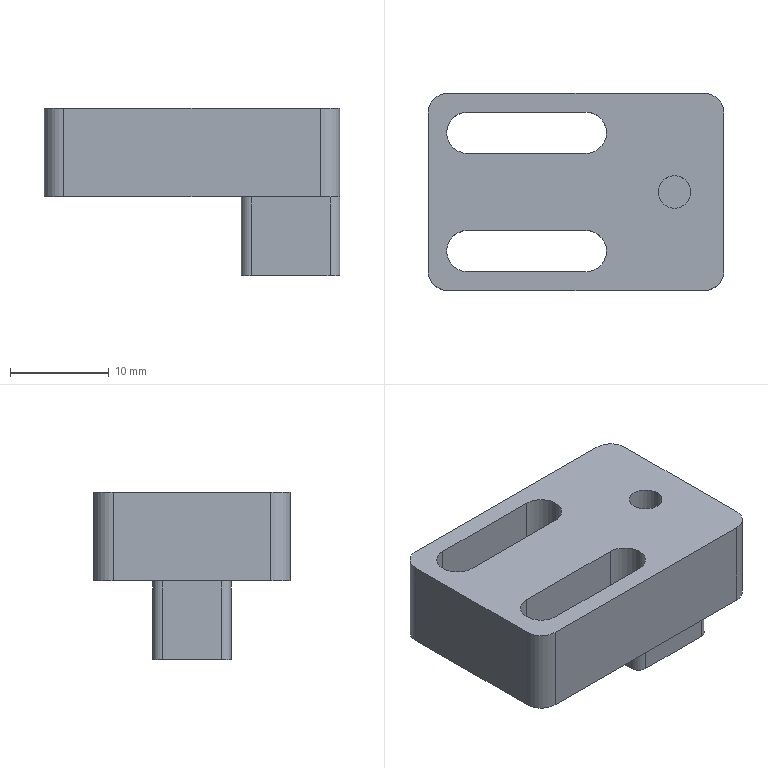Part | SolidWorks | features ICE 5, Fillet 3, Extrusion 1 | 1 solid | 31 faces | box 30 x 20 x 17 mm | volume 4794 mm3 | cylinder 16 | plane 15 | commonest cylinder face diameters 4.2 x6 2 x4 4 x4 3.3 x2
STEP:
#1=CARTESIAN_POINT('',(-9.,8.1,8.));
#2=VERTEX_POINT('',#1);
#3=CARTESIAN_POINT('',(-6.9,6.,8.));
#4=VERTEX_POINT('',#3);
#5=CARTESIAN_POINT('',(-9.,6.,8.));
#6=DIRECTION('',(0.,0.,-1.));
#7=DIRECTION('',(-1.,0.,0.));
#8=AXIS2_PLACEMENT_3D('',#5,#6,#7);
#9=CIRCLE('',#8,2.1);
#10=EDGE_CURVE('',#2,#4,#9,.T.);
#11=ORIENTED_EDGE('',*,*,#10,.T.);
#12=CARTESIAN_POINT('',(-6.9,6.,17.));
#13=VERTEX_POINT('',#12);
#14=CARTESIAN_POINT('',(-6.9,6.,-3.));
#15=DIRECTION('',(0.,0.,1.));
#16=VECTOR('',#15,1000.);
#17=LINE('',#14,#16);
#18=EDGE_CURVE('',#4,#13,#17,.T.);
#19=ORIENTED_EDGE('',*,*,#18,.T.);
#20=CARTESIAN_POINT('',(-9.,8.1,17.));
#21=VERTEX_POINT('',#20);
#22=CARTESIAN_POINT('',(-9.,6.,17.));
#23=DIRECTION('',(0.,0.,1.));
#24=DIRECTION('',(1.,0.,0.));
#25=AXIS2_PLACEMENT_3D('',#22,#23,#24);
#26=CIRCLE('',#25,2.1);
#27=EDGE_CURVE('',#13,#21,#26,.T.);
#28=ORIENTED_EDGE('',*,*,#27,.T.);
#29=CARTESIAN_POINT('',(-9.,8.1,-3.));
#30=DIRECTION('',(0.,0.,1.));
#31=VECTOR('',#30,1000.);
#32=LINE('',#29,#31);
#33=EDGE_CURVE('',#2,#21,#32,.T.);
#34=ORIENTED_EDGE('',*,*,#33,.F.);
#35=EDGE_LOOP('',(#11,#19,#28,#34));
#36=FACE_OUTER_BOUND('',#35,.T.);
#37=CARTESIAN_POINT('',(-9.,6.,-3.));
#38=DIRECTION('',(0.,0.,1.));
#39=DIRECTION('',(1.,0.,0.));
#40=AXIS2_PLACEMENT_3D('',#37,#38,#39);
#41=CYLINDRICAL_SURFACE('',#40,2.1);
#42=ADVANCED_FACE('',(#36),#41,.F.);
#43=CARTESIAN_POINT('',(-9.,-3.9,8.));
#44=VERTEX_POINT('',#43);
#45=CARTESIAN_POINT('',(-6.9,-6.,8.));
#46=VERTEX_POINT('',#45);
#47=CARTESIAN_POINT('',(-9.,-6.,8.));
#48=DIRECTION('',(0.,0.,-1.));
#49=DIRECTION('',(-1.,0.,0.));
#50=AXIS2_PLACEMENT_3D('',#47,#48,#49);
#51=CIRCLE('',#50,2.1);
#52=EDGE_CURVE('',#44,#46,#51,.T.);
#53=ORIENTED_EDGE('',*,*,#52,.T.);
#54=CARTESIAN_POINT('',(-6.9,-6.,17.));
#55=VERTEX_POINT('',#54);
#56=CARTESIAN_POINT('',(-6.9,-6.,-3.));
#57=DIRECTION('',(0.,0.,1.));
#58=VECTOR('',#57,1000.);
#59=LINE('',#56,#58);
#60=EDGE_CURVE('',#46,#55,#59,.T.);
#61=ORIENTED_EDGE('',*,*,#60,.T.);
#62=CARTESIAN_POINT('',(-9.,-3.9,17.));
#63=VERTEX_POINT('',#62);
#64=CARTESIAN_POINT('',(-9.,-6.,17.));
#65=DIRECTION('',(0.,0.,1.));
#66=DIRECTION('',(-1.,0.,0.));
#67=AXIS2_PLACEMENT_3D('',#64,#65,#66);
#68=CIRCLE('',#67,2.1);
#69=EDGE_CURVE('',#55,#63,#68,.T.);
#70=ORIENTED_EDGE('',*,*,#69,.T.);
#71=CARTESIAN_POINT('',(-9.,-3.9,-3.));
#72=DIRECTION('',(0.,0.,1.));
#73=VECTOR('',#72,1000.);
#74=LINE('',#71,#73);
#75=EDGE_CURVE('',#44,#63,#74,.T.);
#76=ORIENTED_EDGE('',*,*,#75,.F.);
#77=EDGE_LOOP('',(#53,#61,#70,#76));
#78=FACE_OUTER_BOUND('',#77,.T.);
#79=CARTESIAN_POINT('',(-9.,-6.,-3.));
#80=DIRECTION('',(0.,0.,1.));
#81=DIRECTION('',(1.,0.,0.));
#82=AXIS2_PLACEMENT_3D('',#79,#80,#81);
#83=CYLINDRICAL_SURFACE('',#82,2.1);
#84=ADVANCED_FACE('',(#78),#83,.F.);
#85=CARTESIAN_POINT('',(-1.65,0.,11.));
#86=VERTEX_POINT('',#85);
#87=CARTESIAN_POINT('',(1.65,0.,11.));
#88=VERTEX_POINT('',#87);
#89=CARTESIAN_POINT('',(0.,0.,11.));
#90=DIRECTION('',(0.,0.,1.));
#91=DIRECTION('',(1.,0.,0.));
#92=AXIS2_PLACEMENT_3D('',#89,#90,#91);
#93=CIRCLE('',#92,1.65);
#94=EDGE_CURVE('',#86,#88,#93,.T.);
#95=ORIENTED_EDGE('',*,*,#94,.F.);
#96=CARTESIAN_POINT('',(-1.65,0.,17.));
#97=VERTEX_POINT('',#96);
#98=CARTESIAN_POINT('',(-1.65,0.,11.));
#99=DIRECTION('',(0.,0.,1.));
#100=VECTOR('',#99,1000.);
#101=LINE('',#98,#100);
#102=EDGE_CURVE('',#86,#97,#101,.T.);
#103=ORIENTED_EDGE('',*,*,#102,.T.);
#104=CARTESIAN_POINT('',(1.65,0.,17.));
#105=VERTEX_POINT('',#104);
#106=CARTESIAN_POINT('',(0.,0.,17.));
#107=DIRECTION('',(0.,0.,1.));
#108=DIRECTION('',(1.,0.,0.));
#109=AXIS2_PLACEMENT_3D('',#106,#107,#108);
#110=CIRCLE('',#109,1.65);
#111=EDGE_CURVE('',#97,#105,#110,.T.);
#112=ORIENTED_EDGE('',*,*,#111,.T.);
#113=CARTESIAN_POINT('',(1.65,0.,11.));
#114=DIRECTION('',(0.,0.,1.));
#115=VECTOR('',#114,1000.);
#116=LINE('',#113,#115);
#117=EDGE_CURVE('',#88,#105,#116,.T.);
#118=ORIENTED_EDGE('',*,*,#117,.F.);
#119=EDGE_LOOP('',(#95,#103,#112,#118));
#120=FACE_OUTER_BOUND('',#119,.T.);
#121=CARTESIAN_POINT('',(0.,0.,11.));
#122=DIRECTION('',(0.,0.,1.));
#123=DIRECTION('',(1.,0.,0.));
#124=AXIS2_PLACEMENT_3D('',#121,#122,#123);
#125=CYLINDRICAL_SURFACE('',#124,1.65);
#126=ADVANCED_FACE('',(#120),#125,.F.);
#127=CARTESIAN_POINT('',(-5.,3.,8.));
#128=VERTEX_POINT('',#127);
#129=CARTESIAN_POINT('',(-5.,-3.,8.));
#130=VERTEX_POINT('',#129);
#131=CARTESIAN_POINT('',(-5.,10.,8.));
#132=DIRECTION('',(0.,-1.,0.));
#133=VECTOR('',#132,1000.);
#134=LINE('',#131,#133);
#135=EDGE_CURVE('',#128,#130,#134,.T.);
#136=ORIENTED_EDGE('',*,*,#135,.F.);
#137=CARTESIAN_POINT('',(-5.,3.,0.));
#138=VERTEX_POINT('',#137);
#139=CARTESIAN_POINT('',(-5.,3.,8.));
#140=DIRECTION('',(0.,0.,-1.));
#141=VECTOR('',#140,1000.);
#142=LINE('',#139,#141);
#143=EDGE_CURVE('',#128,#138,#142,.T.);
#144=ORIENTED_EDGE('',*,*,#143,.T.);
#145=CARTESIAN_POINT('',(-5.,-3.,0.));
#146=VERTEX_POINT('',#145);
#147=CARTESIAN_POINT('',(-5.,-4.,0.));
#148=DIRECTION('',(0.,-1.,0.));
#149=VECTOR('',#148,1000.);
#150=LINE('',#147,#149);
#151=EDGE_CURVE('',#138,#146,#150,.T.);
#152=ORIENTED_EDGE('',*,*,#151,.T.);
#153=CARTESIAN_POINT('',(-5.,-3.,8.));
#154=DIRECTION('',(0.,0.,1.));
#155=VECTOR('',#154,1000.);
#156=LINE('',#153,#155);
#157=EDGE_CURVE('',#146,#130,#156,.T.);
#158=ORIENTED_EDGE('',*,*,#157,.T.);
#159=EDGE_LOOP('',(#136,#144,#152,#158));
#160=FACE_OUTER_BOUND('',#159,.T.);
#161=CARTESIAN_POINT('',(-5.,-4.,8.));
#162=DIRECTION('',(1.,0.,0.));
#163=DIRECTION('',(0.,0.,-1.));
#164=AXIS2_PLACEMENT_3D('',#161,#162,#163);
#165=PLANE('',#164);
#166=ADVANCED_FACE('',(#160),#165,.F.);
#167=CARTESIAN_POINT('',(5.,-3.,0.));
#168=VERTEX_POINT('',#167);
#169=CARTESIAN_POINT('',(5.,3.,0.));
#170=VERTEX_POINT('',#169);
#171=CARTESIAN_POINT('',(5.,-4.,0.));
#172=DIRECTION('',(0.,1.,0.));
#173=VECTOR('',#172,1000.);
#174=LINE('',#171,#173);
#175=EDGE_CURVE('',#168,#170,#174,.T.);
#176=ORIENTED_EDGE('',*,*,#175,.T.);
#177=CARTESIAN_POINT('',(5.,3.,8.));
#178=VERTEX_POINT('',#177);
#179=CARTESIAN_POINT('',(5.,3.,8.));
#180=DIRECTION('',(0.,0.,1.));
#181=VECTOR('',#180,1000.);
#182=LINE('',#179,#181);
#183=EDGE_CURVE('',#170,#178,#182,.T.);
#184=ORIENTED_EDGE('',*,*,#183,.T.);
#185=CARTESIAN_POINT('',(5.,8.,8.));
#186=VERTEX_POINT('',#185);
#187=CARTESIAN_POINT('',(5.,-10.,8.));
#188=DIRECTION('',(0.,1.,0.));
#189=VECTOR('',#188,1000.);
#190=LINE('',#187,#189);
#191=EDGE_CURVE('',#178,#186,#190,.T.);
#192=ORIENTED_EDGE('',*,*,#191,.T.);
#193=CARTESIAN_POINT('',(5.,8.,17.));
#194=VERTEX_POINT('',#193);
#195=CARTESIAN_POINT('',(5.,8.,8.));
#196=DIRECTION('',(0.,0.,1.));
#197=VECTOR('',#196,1000.);
#198=LINE('',#195,#197);
#199=EDGE_CURVE('',#186,#194,#198,.T.);
#200=ORIENTED_EDGE('',*,*,#199,.T.);
#201=CARTESIAN_POINT('',(5.,-8.,17.));
#202=VERTEX_POINT('',#201);
#203=CARTESIAN_POINT('',(5.,-10.,17.));
#204=DIRECTION('',(0.,1.,0.));
#205=VECTOR('',#204,1000.);
#206=LINE('',#203,#205);
#207=EDGE_CURVE('',#202,#194,#206,.T.);
#208=ORIENTED_EDGE('',*,*,#207,.F.);
#209=CARTESIAN_POINT('',(5.,-8.,8.));
#210=VERTEX_POINT('',#209);
#211=CARTESIAN_POINT('',(5.,-8.,8.));
#212=DIRECTION('',(0.,0.,-1.));
#213=VECTOR('',#212,1000.);
#214=LINE('',#211,#213);
#215=EDGE_CURVE('',#202,#210,#214,.T.);
#216=ORIENTED_EDGE('',*,*,#215,.T.);
#217=CARTESIAN_POINT('',(5.,-3.,8.));
#218=VERTEX_POINT('',#217);
#219=CARTESIAN_POINT('',(5.,-10.,8.));
#220=DIRECTION('',(0.,1.,0.));
#221=VECTOR('',#220,1000.);
#222=LINE('',#219,#221);
#223=EDGE_CURVE('',#210,#218,#222,.T.);
#224=ORIENTED_EDGE('',*,*,#223,.T.);
#225=CARTESIAN_POINT('',(5.,-3.,8.));
#226=DIRECTION('',(0.,0.,-1.));
#227=VECTOR('',#226,1000.);
#228=LINE('',#225,#227);
#229=EDGE_CURVE('',#218,#168,#228,.T.);
#230=ORIENTED_EDGE('',*,*,#229,.T.);
#231=EDGE_LOOP('',(#176,#184,#192,#200,#208,#216,#224,#230));
#232=FACE_OUTER_BOUND('',#231,.T.);
#233=CARTESIAN_POINT('',(5.,-4.,8.));
#234=DIRECTION('',(-1.,0.,0.));
#235=DIRECTION('',(0.,0.,1.));
#236=AXIS2_PLACEMENT_3D('',#233,#234,#235);
#237=PLANE('',#236);
#238=ADVANCED_FACE('',(#232),#237,.F.);
#239=CARTESIAN_POINT('',(4.,4.,0.));
#240=VERTEX_POINT('',#239);
#241=CARTESIAN_POINT('',(-4.,4.,0.));
#242=VERTEX_POINT('',#241);
#243=CARTESIAN_POINT('',(-5.,4.,0.));
#244=DIRECTION('',(-1.,0.,0.));
#245=VECTOR('',#244,1000.);
#246=LINE('',#243,#245);
#247=EDGE_CURVE('',#240,#242,#246,.T.);
#248=ORIENTED_EDGE('',*,*,#247,.T.);
#249=CARTESIAN_POINT('',(-4.,4.,8.));
#250=VERTEX_POINT('',#249);
#251=CARTESIAN_POINT('',(-4.,4.,8.));
#252=DIRECTION('',(0.,0.,1.));
#253=VECTOR('',#252,1000.);
#254=LINE('',#251,#253);
#255=EDGE_CURVE('',#242,#250,#254,.T.);
#256=ORIENTED_EDGE('',*,*,#255,.T.);
#257=CARTESIAN_POINT('',(4.,4.,8.));
#258=VERTEX_POINT('',#257);
#259=CARTESIAN_POINT('',(-5.,4.,8.));
#260=DIRECTION('',(-1.,0.,0.));
#261=VECTOR('',#260,1000.);
#262=LINE('',#259,#261);
#263=EDGE_CURVE('',#258,#250,#262,.T.);
#264=ORIENTED_EDGE('',*,*,#263,.F.);
#265=CARTESIAN_POINT('',(4.,4.,8.));
#266=DIRECTION('',(0.,0.,-1.));
#267=VECTOR('',#266,1000.);
#268=LINE('',#265,#267);
#269=EDGE_CURVE('',#258,#240,#268,.T.);
#270=ORIENTED_EDGE('',*,*,#269,.T.);
#271=EDGE_LOOP('',(#248,#256,#264,#270));
#272=FACE_OUTER_BOUND('',#271,.T.);
#273=CARTESIAN_POINT('',(-5.,4.,8.));
#274=DIRECTION('',(0.,-1.,0.));
#275=DIRECTION('',(0.,0.,-1.));
#276=AXIS2_PLACEMENT_3D('',#273,#274,#275);
#277=PLANE('',#276);
#278=ADVANCED_FACE('',(#272),#277,.F.);
#279=CARTESIAN_POINT('',(-4.,-4.,0.));
#280=VERTEX_POINT('',#279);
#281=CARTESIAN_POINT('',(4.,-4.,0.));
#282=VERTEX_POINT('',#281);
#283=CARTESIAN_POINT('',(-5.,-4.,0.));
#284=DIRECTION('',(1.,0.,0.));
#285=VECTOR('',#284,1000.);
#286=LINE('',#283,#285);
#287=EDGE_CURVE('',#280,#282,#286,.T.);
#288=ORIENTED_EDGE('',*,*,#287,.T.);
#289=CARTESIAN_POINT('',(4.,-4.,8.));
#290=VERTEX_POINT('',#289);
#291=CARTESIAN_POINT('',(4.,-4.,8.));
#292=DIRECTION('',(0.,0.,1.));
#293=VECTOR('',#292,1000.);
#294=LINE('',#291,#293);
#295=EDGE_CURVE('',#282,#290,#294,.T.);
#296=ORIENTED_EDGE('',*,*,#295,.T.);
#297=CARTESIAN_POINT('',(-4.,-4.,8.));
#298=VERTEX_POINT('',#297);
#299=CARTESIAN_POINT('',(-5.,-4.,8.));
#300=DIRECTION('',(1.,0.,0.));
#301=VECTOR('',#300,1000.);
#302=LINE('',#299,#301);
#303=EDGE_CURVE('',#298,#290,#302,.T.);
#304=ORIENTED_EDGE('',*,*,#303,.F.);
#305=CARTESIAN_POINT('',(-4.,-4.,8.));
#306=DIRECTION('',(0.,0.,-1.));
#307=VECTOR('',#306,1000.);
#308=LINE('',#305,#307);
#309=EDGE_CURVE('',#298,#280,#308,.T.);
#310=ORIENTED_EDGE('',*,*,#309,.T.);
#311=EDGE_LOOP('',(#288,#296,#304,#310));
#312=FACE_OUTER_BOUND('',#311,.T.);
#313=CARTESIAN_POINT('',(-5.,-4.,8.));
#314=DIRECTION('',(0.,1.,0.));
#315=DIRECTION('',(0.,0.,1.));
#316=AXIS2_PLACEMENT_3D('',#313,#314,#315);
#317=PLANE('',#316);
#318=ADVANCED_FACE('',(#312),#317,.F.);
#319=ORIENTED_EDGE('',*,*,#151,.F.);
#320=CARTESIAN_POINT('',(-4.,3.,0.));
#321=DIRECTION('',(0.,0.,-1.));
#322=DIRECTION('',(-1.,0.,0.));
#323=AXIS2_PLACEMENT_3D('',#320,#321,#322);
#324=CIRCLE('',#323,1.);
#325=EDGE_CURVE('',#138,#242,#324,.T.);
#326=ORIENTED_EDGE('',*,*,#325,.T.);
#327=ORIENTED_EDGE('',*,*,#247,.F.);
#328=CARTESIAN_POINT('',(4.,3.,0.));
#329=DIRECTION('',(0.,0.,-1.));
#330=DIRECTION('',(-1.,0.,0.));
#331=AXIS2_PLACEMENT_3D('',#328,#329,#330);
#332=CIRCLE('',#331,1.);
#333=EDGE_CURVE('',#240,#170,#332,.T.);
#334=ORIENTED_EDGE('',*,*,#333,.T.);
#335=ORIENTED_EDGE('',*,*,#175,.F.);
#336=CARTESIAN_POINT('',(4.,-3.,0.));
#337=DIRECTION('',(0.,0.,-1.));
#338=DIRECTION('',(-1.,0.,0.));
#339=AXIS2_PLACEMENT_3D('',#336,#337,#338);
#340=CIRCLE('',#339,1.);
#341=EDGE_CURVE('',#168,#282,#340,.T.);
#342=ORIENTED_EDGE('',*,*,#341,.T.);
#343=ORIENTED_EDGE('',*,*,#287,.F.);
#344=CARTESIAN_POINT('',(-4.,-3.,0.));
#345=DIRECTION('',(0.,0.,-1.));
#346=DIRECTION('',(-1.,0.,0.));
#347=AXIS2_PLACEMENT_3D('',#344,#345,#346);
#348=CIRCLE('',#347,1.);
#349=EDGE_CURVE('',#280,#146,#348,.T.);
#350=ORIENTED_EDGE('',*,*,#349,.T.);
#351=EDGE_LOOP('',(#319,#326,#327,#334,#335,#342,#343,#350));
#352=FACE_OUTER_BOUND('',#351,.T.);
#353=CARTESIAN_POINT('',(0.,0.,0.));
#354=DIRECTION('',(0.,0.,-1.));
#355=DIRECTION('',(-1.,0.,0.));
#356=AXIS2_PLACEMENT_3D('',#353,#354,#355);
#357=PLANE('',#356);
#358=ADVANCED_FACE('',(#352),#357,.T.);
#359=CARTESIAN_POINT('',(-21.,3.9,8.));
#360=VERTEX_POINT('',#359);
#361=CARTESIAN_POINT('',(-21.,8.1,8.));
#362=VERTEX_POINT('',#361);
#363=CARTESIAN_POINT('',(-21.,6.,8.));
#364=DIRECTION('',(0.,0.,-1.));
#365=DIRECTION('',(-1.,0.,0.));
#366=AXIS2_PLACEMENT_3D('',#363,#364,#365);
#367=CIRCLE('',#366,2.1);
#368=EDGE_CURVE('',#360,#362,#367,.T.);
#369=ORIENTED_EDGE('',*,*,#368,.F.);
#370=CARTESIAN_POINT('',(-9.,3.9,8.));
#371=VERTEX_POINT('',#370);
#372=CARTESIAN_POINT('',(0.,3.9,8.));
#373=DIRECTION('',(-1.,0.,0.));
#374=VECTOR('',#373,1000.);
#375=LINE('',#372,#374);
#376=EDGE_CURVE('',#371,#360,#375,.T.);
#377=ORIENTED_EDGE('',*,*,#376,.F.);
#378=CARTESIAN_POINT('',(-9.,6.,8.));
#379=DIRECTION('',(0.,0.,-1.));
#380=DIRECTION('',(-1.,0.,0.));
#381=AXIS2_PLACEMENT_3D('',#378,#379,#380);
#382=CIRCLE('',#381,2.1);
#383=EDGE_CURVE('',#4,#371,#382,.T.);
#384=ORIENTED_EDGE('',*,*,#383,.F.);
#385=ORIENTED_EDGE('',*,*,#10,.F.);
#386=CARTESIAN_POINT('',(0.,8.1,8.));
#387=DIRECTION('',(1.,0.,0.));
#388=VECTOR('',#387,1000.);
#389=LINE('',#386,#388);
#390=EDGE_CURVE('',#362,#2,#389,.T.);
#391=ORIENTED_EDGE('',*,*,#390,.F.);
#392=EDGE_LOOP('',(#369,#377,#384,#385,#391));
#393=FACE_BOUND('',#392,.T.);
#394=CARTESIAN_POINT('',(-21.,-8.1,8.));
#395=VERTEX_POINT('',#394);
#396=CARTESIAN_POINT('',(-21.,-3.9,8.));
#397=VERTEX_POINT('',#396);
#398=CARTESIAN_POINT('',(-21.,-6.,8.));
#399=DIRECTION('',(0.,0.,-1.));
#400=DIRECTION('',(-1.,0.,0.));
#401=AXIS2_PLACEMENT_3D('',#398,#399,#400);
#402=CIRCLE('',#401,2.1);
#403=EDGE_CURVE('',#395,#397,#402,.T.);
#404=ORIENTED_EDGE('',*,*,#403,.F.);
#405=CARTESIAN_POINT('',(-9.,-8.1,8.));
#406=VERTEX_POINT('',#405);
#407=CARTESIAN_POINT('',(0.,-8.1,8.));
#408=DIRECTION('',(-1.,0.,0.));
#409=VECTOR('',#408,1000.);
#410=LINE('',#407,#409);
#411=EDGE_CURVE('',#406,#395,#410,.T.);
#412=ORIENTED_EDGE('',*,*,#411,.F.);
#413=CARTESIAN_POINT('',(-9.,-6.,8.));
#414=DIRECTION('',(0.,0.,-1.));
#415=DIRECTION('',(-1.,0.,0.));
#416=AXIS2_PLACEMENT_3D('',#413,#414,#415);
#417=CIRCLE('',#416,2.1);
#418=EDGE_CURVE('',#46,#406,#417,.T.);
#419=ORIENTED_EDGE('',*,*,#418,.F.);
#420=ORIENTED_EDGE('',*,*,#52,.F.);
#421=CARTESIAN_POINT('',(0.,-3.9,8.));
#422=DIRECTION('',(1.,0.,0.));
#423=VECTOR('',#422,1000.);
#424=LINE('',#421,#423);
#425=EDGE_CURVE('',#397,#44,#424,.T.);
#426=ORIENTED_EDGE('',*,*,#425,.F.);
#427=EDGE_LOOP('',(#404,#412,#419,#420,#426));
#428=FACE_BOUND('',#427,.T.);
#429=CARTESIAN_POINT('',(3.,10.,8.));
#430=VERTEX_POINT('',#429);
#431=CARTESIAN_POINT('',(-23.,10.,8.));
#432=VERTEX_POINT('',#431);
#433=CARTESIAN_POINT('',(-5.,10.,8.));
#434=DIRECTION('',(-1.,0.,0.));
#435=VECTOR('',#434,1000.);
#436=LINE('',#433,#435);
#437=EDGE_CURVE('',#430,#432,#436,.T.);
#438=ORIENTED_EDGE('',*,*,#437,.F.);
#439=CARTESIAN_POINT('',(3.,8.,8.));
#440=DIRECTION('',(0.,0.,-1.));
#441=DIRECTION('',(-1.,0.,0.));
#442=AXIS2_PLACEMENT_3D('',#439,#440,#441);
#443=CIRCLE('',#442,2.);
#444=EDGE_CURVE('',#430,#186,#443,.T.);
#445=ORIENTED_EDGE('',*,*,#444,.T.);
#446=ORIENTED_EDGE('',*,*,#191,.F.);
#447=CARTESIAN_POINT('',(4.,3.,8.));
#448=DIRECTION('',(0.,0.,1.));
#449=DIRECTION('',(-1.,0.,0.));
#450=AXIS2_PLACEMENT_3D('',#447,#448,#449);
#451=CIRCLE('',#450,1.);
#452=EDGE_CURVE('',#178,#258,#451,.T.);
#453=ORIENTED_EDGE('',*,*,#452,.T.);
#454=ORIENTED_EDGE('',*,*,#263,.T.);
#455=CARTESIAN_POINT('',(-4.,3.,8.));
#456=DIRECTION('',(0.,0.,1.));
#457=DIRECTION('',(-1.,0.,0.));
#458=AXIS2_PLACEMENT_3D('',#455,#456,#457);
#459=CIRCLE('',#458,1.);
#460=EDGE_CURVE('',#250,#128,#459,.T.);
#461=ORIENTED_EDGE('',*,*,#460,.T.);
#462=ORIENTED_EDGE('',*,*,#135,.T.);
#463=CARTESIAN_POINT('',(-4.,-3.,8.));
#464=DIRECTION('',(0.,0.,1.));
#465=DIRECTION('',(-1.,0.,0.));
#466=AXIS2_PLACEMENT_3D('',#463,#464,#465);
#467=CIRCLE('',#466,1.);
#468=EDGE_CURVE('',#130,#298,#467,.T.);
#469=ORIENTED_EDGE('',*,*,#468,.T.);
#470=ORIENTED_EDGE('',*,*,#303,.T.);
#471=CARTESIAN_POINT('',(4.,-3.,8.));
#472=DIRECTION('',(0.,0.,1.));
#473=DIRECTION('',(-1.,0.,0.));
#474=AXIS2_PLACEMENT_3D('',#471,#472,#473);
#475=CIRCLE('',#474,1.);
#476=EDGE_CURVE('',#290,#218,#475,.T.);
#477=ORIENTED_EDGE('',*,*,#476,.T.);
#478=ORIENTED_EDGE('',*,*,#223,.F.);
#479=CARTESIAN_POINT('',(3.,-10.,8.));
#480=VERTEX_POINT('',#479);
#481=CARTESIAN_POINT('',(3.,-8.,8.));
#482=DIRECTION('',(0.,0.,-1.));
#483=DIRECTION('',(-1.,0.,0.));
#484=AXIS2_PLACEMENT_3D('',#481,#482,#483);
#485=CIRCLE('',#484,2.);
#486=EDGE_CURVE('',#210,#480,#485,.T.);
#487=ORIENTED_EDGE('',*,*,#486,.T.);
#488=CARTESIAN_POINT('',(-23.,-10.,8.));
#489=VERTEX_POINT('',#488);
#490=CARTESIAN_POINT('',(-5.,-10.,8.));
#491=DIRECTION('',(1.,0.,0.));
#492=VECTOR('',#491,1000.);
#493=LINE('',#490,#492);
#494=EDGE_CURVE('',#489,#480,#493,.T.);
#495=ORIENTED_EDGE('',*,*,#494,.F.);
#496=CARTESIAN_POINT('',(-25.,-8.,8.));
#497=VERTEX_POINT('',#496);
#498=CARTESIAN_POINT('',(-23.,-8.,8.));
#499=DIRECTION('',(0.,0.,-1.));
#500=DIRECTION('',(-1.,0.,0.));
#501=AXIS2_PLACEMENT_3D('',#498,#499,#500);
#502=CIRCLE('',#501,2.);
#503=EDGE_CURVE('',#489,#497,#502,.T.);
#504=ORIENTED_EDGE('',*,*,#503,.T.);
#505=CARTESIAN_POINT('',(-25.,8.,8.));
#506=VERTEX_POINT('',#505);
#507=CARTESIAN_POINT('',(-25.,10.,8.));
#508=DIRECTION('',(0.,-1.,0.));
#509=VECTOR('',#508,1000.);
#510=LINE('',#507,#509);
#511=EDGE_CURVE('',#506,#497,#510,.T.);
#512=ORIENTED_EDGE('',*,*,#511,.F.);
#513=CARTESIAN_POINT('',(-23.,8.,8.));
#514=DIRECTION('',(0.,0.,-1.));
#515=DIRECTION('',(-1.,0.,0.));
#516=AXIS2_PLACEMENT_3D('',#513,#514,#515);
#517=CIRCLE('',#516,2.);
#518=EDGE_CURVE('',#506,#432,#517,.T.);
#519=ORIENTED_EDGE('',*,*,#518,.T.);
#520=EDGE_LOOP('',(#438,#445,#446,#453,#454,#461,#462,#469,#470,#477,#478,#487,#495,#504,#512,#519));
#521=FACE_OUTER_BOUND('',#520,.T.);
#522=CARTESIAN_POINT('',(0.,0.,8.));
#523=DIRECTION('',(0.,0.,-1.));
#524=DIRECTION('',(-1.,0.,0.));
#525=AXIS2_PLACEMENT_3D('',#522,#523,#524);
#526=PLANE('',#525);
#527=ADVANCED_FACE('',(#393,#428,#521),#526,.T.);
#528=CARTESIAN_POINT('',(3.,10.,17.));
#529=VERTEX_POINT('',#528);
#530=CARTESIAN_POINT('',(-23.,10.,17.));
#531=VERTEX_POINT('',#530);
#532=CARTESIAN_POINT('',(-5.,10.,17.));
#533=DIRECTION('',(-1.,0.,0.));
#534=VECTOR('',#533,1000.);
#535=LINE('',#532,#534);
#536=EDGE_CURVE('',#529,#531,#535,.T.);
#537=ORIENTED_EDGE('',*,*,#536,.F.);
#538=CARTESIAN_POINT('',(3.,10.,17.));
#539=DIRECTION('',(0.,0.,-1.));
#540=VECTOR('',#539,1000.);
#541=LINE('',#538,#540);
#542=EDGE_CURVE('',#529,#430,#541,.T.);
#543=ORIENTED_EDGE('',*,*,#542,.T.);
#544=ORIENTED_EDGE('',*,*,#437,.T.);
#545=CARTESIAN_POINT('',(-23.,10.,17.));
#546=DIRECTION('',(0.,0.,1.));
#547=VECTOR('',#546,1000.);
#548=LINE('',#545,#547);
#549=EDGE_CURVE('',#432,#531,#548,.T.);
#550=ORIENTED_EDGE('',*,*,#549,.T.);
#551=EDGE_LOOP('',(#537,#543,#544,#550));
#552=FACE_OUTER_BOUND('',#551,.T.);
#553=CARTESIAN_POINT('',(-5.,10.,17.));
#554=DIRECTION('',(0.,-1.,0.));
#555=DIRECTION('',(0.,0.,-1.));
#556=AXIS2_PLACEMENT_3D('',#553,#554,#555);
#557=PLANE('',#556);
#558=ADVANCED_FACE('',(#552),#557,.F.);
#559=ORIENTED_EDGE('',*,*,#494,.T.);
#560=CARTESIAN_POINT('',(3.,-10.,17.));
#561=VERTEX_POINT('',#560);
#562=CARTESIAN_POINT('',(3.,-10.,17.));
#563=DIRECTION('',(0.,0.,1.));
#564=VECTOR('',#563,1000.);
#565=LINE('',#562,#564);
#566=EDGE_CURVE('',#480,#561,#565,.T.);
#567=ORIENTED_EDGE('',*,*,#566,.T.);
#568=CARTESIAN_POINT('',(-23.,-10.,17.));
#569=VERTEX_POINT('',#568);
#570=CARTESIAN_POINT('',(-5.,-10.,17.));
#571=DIRECTION('',(1.,0.,0.));
#572=VECTOR('',#571,1000.);
#573=LINE('',#570,#572);
#574=EDGE_CURVE('',#569,#561,#573,.T.);
#575=ORIENTED_EDGE('',*,*,#574,.F.);
#576=CARTESIAN_POINT('',(-23.,-10.,8.));
#577=DIRECTION('',(0.,0.,-1.));
#578=VECTOR('',#577,1000.);
#579=LINE('',#576,#578);
#580=EDGE_CURVE('',#569,#489,#579,.T.);
#581=ORIENTED_EDGE('',*,*,#580,.T.);
#582=EDGE_LOOP('',(#559,#567,#575,#581));
#583=FACE_OUTER_BOUND('',#582,.T.);
#584=CARTESIAN_POINT('',(-5.,-10.,17.));
#585=DIRECTION('',(0.,1.,0.));
#586=DIRECTION('',(0.,0.,1.));
#587=AXIS2_PLACEMENT_3D('',#584,#585,#586);
#588=PLANE('',#587);
#589=ADVANCED_FACE('',(#583),#588,.F.);
#590=CARTESIAN_POINT('',(-21.,3.9,17.));
#591=VERTEX_POINT('',#590);
#592=CARTESIAN_POINT('',(-9.,3.9,17.));
#593=VERTEX_POINT('',#592);
#594=CARTESIAN_POINT('',(-21.,3.9,17.));
#595=DIRECTION('',(1.,0.,0.));
#596=VECTOR('',#595,1000.);
#597=LINE('',#594,#596);
#598=EDGE_CURVE('',#591,#593,#597,.T.);
#599=ORIENTED_EDGE('',*,*,#598,.F.);
#600=CARTESIAN_POINT('',(-21.,8.1,17.));
#601=VERTEX_POINT('',#600);
#602=CARTESIAN_POINT('',(-21.,6.,17.));
#603=DIRECTION('',(0.,0.,1.));
#604=DIRECTION('',(1.,0.,0.));
#605=AXIS2_PLACEMENT_3D('',#602,#603,#604);
#606=CIRCLE('',#605,2.1);
#607=EDGE_CURVE('',#601,#591,#606,.T.);
#608=ORIENTED_EDGE('',*,*,#607,.F.);
#609=CARTESIAN_POINT('',(-21.,8.1,17.));
#610=DIRECTION('',(-1.,0.,0.));
#611=VECTOR('',#610,1000.);
#612=LINE('',#609,#611);
#613=EDGE_CURVE('',#21,#601,#612,.T.);
#614=ORIENTED_EDGE('',*,*,#613,.F.);
#615=ORIENTED_EDGE('',*,*,#27,.F.);
#616=CARTESIAN_POINT('',(-9.,6.,17.));
#617=DIRECTION('',(0.,0.,1.));
#618=DIRECTION('',(1.,0.,0.));
#619=AXIS2_PLACEMENT_3D('',#616,#617,#618);
#620=CIRCLE('',#619,2.1);
#621=EDGE_CURVE('',#593,#13,#620,.T.);
#622=ORIENTED_EDGE('',*,*,#621,.F.);
#623=EDGE_LOOP('',(#599,#608,#614,#615,#622));
#624=FACE_BOUND('',#623,.T.);
#625=CARTESIAN_POINT('',(-21.,-8.1,17.));
#626=VERTEX_POINT('',#625);
#627=CARTESIAN_POINT('',(-9.,-8.1,17.));
#628=VERTEX_POINT('',#627);
#629=CARTESIAN_POINT('',(-21.,-8.1,17.));
#630=DIRECTION('',(1.,0.,0.));
#631=VECTOR('',#630,1000.);
#632=LINE('',#629,#631);
#633=EDGE_CURVE('',#626,#628,#632,.T.);
#634=ORIENTED_EDGE('',*,*,#633,.F.);
#635=CARTESIAN_POINT('',(-21.,-3.9,17.));
#636=VERTEX_POINT('',#635);
#637=CARTESIAN_POINT('',(-21.,-6.,17.));
#638=DIRECTION('',(0.,0.,1.));
#639=DIRECTION('',(-1.,0.,0.));
#640=AXIS2_PLACEMENT_3D('',#637,#638,#639);
#641=CIRCLE('',#640,2.1);
#642=EDGE_CURVE('',#636,#626,#641,.T.);
#643=ORIENTED_EDGE('',*,*,#642,.F.);
#644=CARTESIAN_POINT('',(-21.,-3.9,17.));
#645=DIRECTION('',(-1.,0.,0.));
#646=VECTOR('',#645,1000.);
#647=LINE('',#644,#646);
#648=EDGE_CURVE('',#63,#636,#647,.T.);
#649=ORIENTED_EDGE('',*,*,#648,.F.);
#650=ORIENTED_EDGE('',*,*,#69,.F.);
#651=CARTESIAN_POINT('',(-9.,-6.,17.));
#652=DIRECTION('',(0.,0.,1.));
#653=DIRECTION('',(-1.,0.,0.));
#654=AXIS2_PLACEMENT_3D('',#651,#652,#653);
#655=CIRCLE('',#654,2.1);
#656=EDGE_CURVE('',#628,#55,#655,.T.);
#657=ORIENTED_EDGE('',*,*,#656,.F.);
#658=EDGE_LOOP('',(#634,#643,#649,#650,#657));
#659=FACE_BOUND('',#658,.T.);
#660=CARTESIAN_POINT('',(0.,0.,17.));
#661=DIRECTION('',(0.,0.,1.));
#662=DIRECTION('',(1.,0.,0.));
#663=AXIS2_PLACEMENT_3D('',#660,#661,#662);
#664=CIRCLE('',#663,1.65);
#665=EDGE_CURVE('',#105,#97,#664,.T.);
#666=ORIENTED_EDGE('',*,*,#665,.F.);
#667=ORIENTED_EDGE('',*,*,#111,.F.);
#668=EDGE_LOOP('',(#666,#667));
#669=FACE_BOUND('',#668,.T.);
#670=ORIENTED_EDGE('',*,*,#207,.T.);
#671=CARTESIAN_POINT('',(3.,8.,17.));
#672=DIRECTION('',(0.,0.,1.));
#673=DIRECTION('',(-1.,0.,0.));
#674=AXIS2_PLACEMENT_3D('',#671,#672,#673);
#675=CIRCLE('',#674,2.);
#676=EDGE_CURVE('',#194,#529,#675,.T.);
#677=ORIENTED_EDGE('',*,*,#676,.T.);
#678=ORIENTED_EDGE('',*,*,#536,.T.);
#679=CARTESIAN_POINT('',(-25.,8.,17.));
#680=VERTEX_POINT('',#679);
#681=CARTESIAN_POINT('',(-23.,8.,17.));
#682=DIRECTION('',(0.,0.,1.));
#683=DIRECTION('',(-1.,0.,0.));
#684=AXIS2_PLACEMENT_3D('',#681,#682,#683);
#685=CIRCLE('',#684,2.);
#686=EDGE_CURVE('',#531,#680,#685,.T.);
#687=ORIENTED_EDGE('',*,*,#686,.T.);
#688=CARTESIAN_POINT('',(-25.,-8.,17.));
#689=VERTEX_POINT('',#688);
#690=CARTESIAN_POINT('',(-25.,10.,17.));
#691=DIRECTION('',(0.,1.,0.));
#692=VECTOR('',#691,1000.);
#693=LINE('',#690,#692);
#694=EDGE_CURVE('',#689,#680,#693,.T.);
#695=ORIENTED_EDGE('',*,*,#694,.F.);
#696=CARTESIAN_POINT('',(-23.,-8.,17.));
#697=DIRECTION('',(0.,0.,1.));
#698=DIRECTION('',(-1.,0.,0.));
#699=AXIS2_PLACEMENT_3D('',#696,#697,#698);
#700=CIRCLE('',#699,2.);
#701=EDGE_CURVE('',#689,#569,#700,.T.);
#702=ORIENTED_EDGE('',*,*,#701,.T.);
#703=ORIENTED_EDGE('',*,*,#574,.T.);
#704=CARTESIAN_POINT('',(3.,-8.,17.));
#705=DIRECTION('',(0.,0.,1.));
#706=DIRECTION('',(-1.,0.,0.));
#707=AXIS2_PLACEMENT_3D('',#704,#705,#706);
#708=CIRCLE('',#707,2.);
#709=EDGE_CURVE('',#561,#202,#708,.T.);
#710=ORIENTED_EDGE('',*,*,#709,.T.);
#711=EDGE_LOOP('',(#670,#677,#678,#687,#695,#702,#703,#710));
#712=FACE_OUTER_BOUND('',#711,.T.);
#713=CARTESIAN_POINT('',(0.,0.,17.));
#714=DIRECTION('',(0.,0.,-1.));
#715=DIRECTION('',(-1.,0.,0.));
#716=AXIS2_PLACEMENT_3D('',#713,#714,#715);
#717=PLANE('',#716);
#718=ADVANCED_FACE('',(#624,#659,#669,#712),#717,.F.);
#719=ORIENTED_EDGE('',*,*,#102,.F.);
#720=CARTESIAN_POINT('',(0.,0.,11.));
#721=DIRECTION('',(0.,0.,1.));
#722=DIRECTION('',(1.,0.,0.));
#723=AXIS2_PLACEMENT_3D('',#720,#721,#722);
#724=CIRCLE('',#723,1.65);
#725=EDGE_CURVE('',#88,#86,#724,.T.);
#726=ORIENTED_EDGE('',*,*,#725,.F.);
#727=ORIENTED_EDGE('',*,*,#117,.T.);
#728=ORIENTED_EDGE('',*,*,#665,.T.);
#729=EDGE_LOOP('',(#719,#726,#727,#728));
#730=FACE_OUTER_BOUND('',#729,.T.);
#731=CARTESIAN_POINT('',(0.,0.,11.));
#732=DIRECTION('',(0.,0.,1.));
#733=DIRECTION('',(1.,0.,0.));
#734=AXIS2_PLACEMENT_3D('',#731,#732,#733);
#735=CYLINDRICAL_SURFACE('',#734,1.65);
#736=ADVANCED_FACE('',(#730),#735,.F.);
#737=ORIENTED_EDGE('',*,*,#725,.T.);
#738=ORIENTED_EDGE('',*,*,#94,.T.);
#739=EDGE_LOOP('',(#737,#738));
#740=FACE_OUTER_BOUND('',#739,.T.);
#741=CARTESIAN_POINT('',(0.,0.,11.));
#742=DIRECTION('',(0.,0.,1.));
#743=DIRECTION('',(1.,0.,0.));
#744=AXIS2_PLACEMENT_3D('',#741,#742,#743);
#745=PLANE('',#744);
#746=ADVANCED_FACE('',(#740),#745,.T.);
#747=ORIENTED_EDGE('',*,*,#511,.T.);
#748=CARTESIAN_POINT('',(-25.,-8.,17.));
#749=DIRECTION('',(0.,0.,1.));
#750=VECTOR('',#749,1000.);
#751=LINE('',#748,#750);
#752=EDGE_CURVE('',#497,#689,#751,.T.);
#753=ORIENTED_EDGE('',*,*,#752,.T.);
#754=ORIENTED_EDGE('',*,*,#694,.T.);
#755=CARTESIAN_POINT('',(-25.,8.,8.));
#756=DIRECTION('',(0.,0.,-1.));
#757=VECTOR('',#756,1000.);
#758=LINE('',#755,#757);
#759=EDGE_CURVE('',#680,#506,#758,.T.);
#760=ORIENTED_EDGE('',*,*,#759,.T.);
#761=EDGE_LOOP('',(#747,#753,#754,#760));
#762=FACE_OUTER_BOUND('',#761,.T.);
#763=CARTESIAN_POINT('',(-25.,0.,0.));
#764=DIRECTION('',(-1.,0.,0.));
#765=DIRECTION('',(0.,0.,1.));
#766=AXIS2_PLACEMENT_3D('',#763,#764,#765);
#767=PLANE('',#766);
#768=ADVANCED_FACE('',(#762),#767,.T.);
#769=ORIENTED_EDGE('',*,*,#403,.T.);
#770=CARTESIAN_POINT('',(-21.,-3.9,-3.));
#771=DIRECTION('',(0.,0.,1.));
#772=VECTOR('',#771,1000.);
#773=LINE('',#770,#772);
#774=EDGE_CURVE('',#397,#636,#773,.T.);
#775=ORIENTED_EDGE('',*,*,#774,.T.);
#776=ORIENTED_EDGE('',*,*,#642,.T.);
#777=CARTESIAN_POINT('',(-21.,-8.1,-3.));
#778=DIRECTION('',(0.,0.,1.));
#779=VECTOR('',#778,1000.);
#780=LINE('',#777,#779);
#781=EDGE_CURVE('',#395,#626,#780,.T.);
#782=ORIENTED_EDGE('',*,*,#781,.F.);
#783=EDGE_LOOP('',(#769,#775,#776,#782));
#784=FACE_OUTER_BOUND('',#783,.T.);
#785=CARTESIAN_POINT('',(-21.,-6.,-3.));
#786=DIRECTION('',(0.,0.,1.));
#787=DIRECTION('',(1.,0.,0.));
#788=AXIS2_PLACEMENT_3D('',#785,#786,#787);
#789=CYLINDRICAL_SURFACE('',#788,2.1);
#790=ADVANCED_FACE('',(#784),#789,.F.);
#791=ORIENTED_EDGE('',*,*,#425,.T.);
#792=ORIENTED_EDGE('',*,*,#75,.T.);
#793=ORIENTED_EDGE('',*,*,#648,.T.);
#794=ORIENTED_EDGE('',*,*,#774,.F.);
#795=EDGE_LOOP('',(#791,#792,#793,#794));
#796=FACE_OUTER_BOUND('',#795,.T.);
#797=CARTESIAN_POINT('',(-21.,-3.9,-3.));
#798=DIRECTION('',(0.,1.,0.));
#799=DIRECTION('',(-1.,0.,0.));
#800=AXIS2_PLACEMENT_3D('',#797,#798,#799);
#801=PLANE('',#800);
#802=ADVANCED_FACE('',(#796),#801,.F.);
#803=ORIENTED_EDGE('',*,*,#60,.F.);
#804=ORIENTED_EDGE('',*,*,#418,.T.);
#805=CARTESIAN_POINT('',(-9.,-8.1,-3.));
#806=DIRECTION('',(0.,0.,1.));
#807=VECTOR('',#806,1000.);
#808=LINE('',#805,#807);
#809=EDGE_CURVE('',#406,#628,#808,.T.);
#810=ORIENTED_EDGE('',*,*,#809,.T.);
#811=ORIENTED_EDGE('',*,*,#656,.T.);
#812=EDGE_LOOP('',(#803,#804,#810,#811));
#813=FACE_OUTER_BOUND('',#812,.T.);
#814=CARTESIAN_POINT('',(-9.,-6.,-3.));
#815=DIRECTION('',(0.,0.,1.));
#816=DIRECTION('',(1.,0.,0.));
#817=AXIS2_PLACEMENT_3D('',#814,#815,#816);
#818=CYLINDRICAL_SURFACE('',#817,2.1);
#819=ADVANCED_FACE('',(#813),#818,.F.);
#820=ORIENTED_EDGE('',*,*,#411,.T.);
#821=ORIENTED_EDGE('',*,*,#781,.T.);
#822=ORIENTED_EDGE('',*,*,#633,.T.);
#823=ORIENTED_EDGE('',*,*,#809,.F.);
#824=EDGE_LOOP('',(#820,#821,#822,#823));
#825=FACE_OUTER_BOUND('',#824,.T.);
#826=CARTESIAN_POINT('',(-21.,-8.1,-3.));
#827=DIRECTION('',(0.,-1.,0.));
#828=DIRECTION('',(0.,0.,-1.));
#829=AXIS2_PLACEMENT_3D('',#826,#827,#828);
#830=PLANE('',#829);
#831=ADVANCED_FACE('',(#825),#830,.F.);
#832=ORIENTED_EDGE('',*,*,#368,.T.);
#833=CARTESIAN_POINT('',(-21.,8.1,-3.));
#834=DIRECTION('',(0.,0.,1.));
#835=VECTOR('',#834,1000.);
#836=LINE('',#833,#835);
#837=EDGE_CURVE('',#362,#601,#836,.T.);
#838=ORIENTED_EDGE('',*,*,#837,.T.);
#839=ORIENTED_EDGE('',*,*,#607,.T.);
#840=CARTESIAN_POINT('',(-21.,3.9,-3.));
#841=DIRECTION('',(0.,0.,1.));
#842=VECTOR('',#841,1000.);
#843=LINE('',#840,#842);
#844=EDGE_CURVE('',#360,#591,#843,.T.);
#845=ORIENTED_EDGE('',*,*,#844,.F.);
#846=EDGE_LOOP('',(#832,#838,#839,#845));
#847=FACE_OUTER_BOUND('',#846,.T.);
#848=CARTESIAN_POINT('',(-21.,6.,-3.));
#849=DIRECTION('',(0.,0.,1.));
#850=DIRECTION('',(1.,0.,0.));
#851=AXIS2_PLACEMENT_3D('',#848,#849,#850);
#852=CYLINDRICAL_SURFACE('',#851,2.1);
#853=ADVANCED_FACE('',(#847),#852,.F.);
#854=ORIENTED_EDGE('',*,*,#390,.T.);
#855=ORIENTED_EDGE('',*,*,#33,.T.);
#856=ORIENTED_EDGE('',*,*,#613,.T.);
#857=ORIENTED_EDGE('',*,*,#837,.F.);
#858=EDGE_LOOP('',(#854,#855,#856,#857));
#859=FACE_OUTER_BOUND('',#858,.T.);
#860=CARTESIAN_POINT('',(-21.,8.1,-3.));
#861=DIRECTION('',(0.,1.,0.));
#862=DIRECTION('',(0.,0.,1.));
#863=AXIS2_PLACEMENT_3D('',#860,#861,#862);
#864=PLANE('',#863);
#865=ADVANCED_FACE('',(#859),#864,.F.);
#866=ORIENTED_EDGE('',*,*,#18,.F.);
#867=ORIENTED_EDGE('',*,*,#383,.T.);
#868=CARTESIAN_POINT('',(-9.,3.9,-3.));
#869=DIRECTION('',(0.,0.,1.));
#870=VECTOR('',#869,1000.);
#871=LINE('',#868,#870);
#872=EDGE_CURVE('',#371,#593,#871,.T.);
#873=ORIENTED_EDGE('',*,*,#872,.T.);
#874=ORIENTED_EDGE('',*,*,#621,.T.);
#875=EDGE_LOOP('',(#866,#867,#873,#874));
#876=FACE_OUTER_BOUND('',#875,.T.);
#877=CARTESIAN_POINT('',(-9.,6.,-3.));
#878=DIRECTION('',(0.,0.,1.));
#879=DIRECTION('',(1.,0.,0.));
#880=AXIS2_PLACEMENT_3D('',#877,#878,#879);
#881=CYLINDRICAL_SURFACE('',#880,2.1);
#882=ADVANCED_FACE('',(#876),#881,.F.);
#883=ORIENTED_EDGE('',*,*,#376,.T.);
#884=ORIENTED_EDGE('',*,*,#844,.T.);
#885=ORIENTED_EDGE('',*,*,#598,.T.);
#886=ORIENTED_EDGE('',*,*,#872,.F.);
#887=EDGE_LOOP('',(#883,#884,#885,#886));
#888=FACE_OUTER_BOUND('',#887,.T.);
#889=CARTESIAN_POINT('',(-21.,3.9,-3.));
#890=DIRECTION('',(0.,-1.,0.));
#891=DIRECTION('',(0.,0.,-1.));
#892=AXIS2_PLACEMENT_3D('',#889,#890,#891);
#893=PLANE('',#892);
#894=ADVANCED_FACE('',(#888),#893,.F.);
#895=ORIENTED_EDGE('',*,*,#676,.F.);
#896=ORIENTED_EDGE('',*,*,#199,.F.);
#897=ORIENTED_EDGE('',*,*,#444,.F.);
#898=ORIENTED_EDGE('',*,*,#542,.F.);
#899=EDGE_LOOP('',(#895,#896,#897,#898));
#900=FACE_OUTER_BOUND('',#899,.T.);
#901=CARTESIAN_POINT('',(3.,8.,17.));
#902=DIRECTION('',(0.,0.,-1.));
#903=DIRECTION('',(-1.,0.,0.));
#904=AXIS2_PLACEMENT_3D('',#901,#902,#903);
#905=CYLINDRICAL_SURFACE('',#904,2.);
#906=ADVANCED_FACE('',(#900),#905,.T.);
#907=ORIENTED_EDGE('',*,*,#709,.F.);
#908=ORIENTED_EDGE('',*,*,#566,.F.);
#909=ORIENTED_EDGE('',*,*,#486,.F.);
#910=ORIENTED_EDGE('',*,*,#215,.F.);
#911=EDGE_LOOP('',(#907,#908,#909,#910));
#912=FACE_OUTER_BOUND('',#911,.T.);
#913=CARTESIAN_POINT('',(3.,-8.,8.));
#914=DIRECTION('',(0.,0.,-1.));
#915=DIRECTION('',(-1.,0.,0.));
#916=AXIS2_PLACEMENT_3D('',#913,#914,#915);
#917=CYLINDRICAL_SURFACE('',#916,2.);
#918=ADVANCED_FACE('',(#912),#917,.T.);
#919=ORIENTED_EDGE('',*,*,#503,.F.);
#920=ORIENTED_EDGE('',*,*,#580,.F.);
#921=ORIENTED_EDGE('',*,*,#701,.F.);
#922=ORIENTED_EDGE('',*,*,#752,.F.);
#923=EDGE_LOOP('',(#919,#920,#921,#922));
#924=FACE_OUTER_BOUND('',#923,.T.);
#925=CARTESIAN_POINT('',(-23.,-8.,0.));
#926=DIRECTION('',(0.,0.,-1.));
#927=DIRECTION('',(-1.,0.,0.));
#928=AXIS2_PLACEMENT_3D('',#925,#926,#927);
#929=CYLINDRICAL_SURFACE('',#928,2.);
#930=ADVANCED_FACE('',(#924),#929,.T.);
#931=ORIENTED_EDGE('',*,*,#686,.F.);
#932=ORIENTED_EDGE('',*,*,#549,.F.);
#933=ORIENTED_EDGE('',*,*,#518,.F.);
#934=ORIENTED_EDGE('',*,*,#759,.F.);
#935=EDGE_LOOP('',(#931,#932,#933,#934));
#936=FACE_OUTER_BOUND('',#935,.T.);
#937=CARTESIAN_POINT('',(-23.,8.,0.));
#938=DIRECTION('',(0.,0.,1.));
#939=DIRECTION('',(1.,0.,0.));
#940=AXIS2_PLACEMENT_3D('',#937,#938,#939);
#941=CYLINDRICAL_SURFACE('',#940,2.);
#942=ADVANCED_FACE('',(#936),#941,.T.);
#943=ORIENTED_EDGE('',*,*,#460,.F.);
#944=ORIENTED_EDGE('',*,*,#255,.F.);
#945=ORIENTED_EDGE('',*,*,#325,.F.);
#946=ORIENTED_EDGE('',*,*,#143,.F.);
#947=EDGE_LOOP('',(#943,#944,#945,#946));
#948=FACE_OUTER_BOUND('',#947,.T.);
#949=CARTESIAN_POINT('',(-4.,3.,8.));
#950=DIRECTION('',(0.,0.,-1.));
#951=DIRECTION('',(-1.,0.,0.));
#952=AXIS2_PLACEMENT_3D('',#949,#950,#951);
#953=CYLINDRICAL_SURFACE('',#952,1.);
#954=ADVANCED_FACE('',(#948),#953,.T.);
#955=ORIENTED_EDGE('',*,*,#452,.F.);
#956=ORIENTED_EDGE('',*,*,#183,.F.);
#957=ORIENTED_EDGE('',*,*,#333,.F.);
#958=ORIENTED_EDGE('',*,*,#269,.F.);
#959=EDGE_LOOP('',(#955,#956,#957,#958));
#960=FACE_OUTER_BOUND('',#959,.T.);
#961=CARTESIAN_POINT('',(4.,3.,8.));
#962=DIRECTION('',(0.,0.,-1.));
#963=DIRECTION('',(-1.,0.,0.));
#964=AXIS2_PLACEMENT_3D('',#961,#962,#963);
#965=CYLINDRICAL_SURFACE('',#964,1.);
#966=ADVANCED_FACE('',(#960),#965,.T.);
#967=ORIENTED_EDGE('',*,*,#476,.F.);
#968=ORIENTED_EDGE('',*,*,#295,.F.);
#969=ORIENTED_EDGE('',*,*,#341,.F.);
#970=ORIENTED_EDGE('',*,*,#229,.F.);
#971=EDGE_LOOP('',(#967,#968,#969,#970));
#972=FACE_OUTER_BOUND('',#971,.T.);
#973=CARTESIAN_POINT('',(4.,-3.,8.));
#974=DIRECTION('',(0.,0.,-1.));
#975=DIRECTION('',(-1.,0.,0.));
#976=AXIS2_PLACEMENT_3D('',#973,#974,#975);
#977=CYLINDRICAL_SURFACE('',#976,1.);
#978=ADVANCED_FACE('',(#972),#977,.T.);
#979=ORIENTED_EDGE('',*,*,#468,.F.);
#980=ORIENTED_EDGE('',*,*,#157,.F.);
#981=ORIENTED_EDGE('',*,*,#349,.F.);
#982=ORIENTED_EDGE('',*,*,#309,.F.);
#983=EDGE_LOOP('',(#979,#980,#981,#982));
#984=FACE_OUTER_BOUND('',#983,.T.);
#985=CARTESIAN_POINT('',(-4.,-3.,8.));
#986=DIRECTION('',(0.,0.,-1.));
#987=DIRECTION('',(-1.,0.,0.));
#988=AXIS2_PLACEMENT_3D('',#985,#986,#987);
#989=CYLINDRICAL_SURFACE('',#988,1.);
#990=ADVANCED_FACE('',(#984),#989,.T.);
#991=CLOSED_SHELL('',(#42,#84,#126,#166,#238,#278,#318,#358,#527,#558,#589,#718,#736,#746,#768,#790,#802,#819,#831,#853,#865,#882,#894,#906,#918,#930,#942,#954,#966,#978,#990));
#992=MANIFOLD_SOLID_BREP('',#991);
#993=CARTESIAN_POINT('',(0.,0.,0.));
#994=DIRECTION('',(0.,0.,1.));
#995=DIRECTION('',(1.,0.,0.));
#996=AXIS2_PLACEMENT_3D('',#993,#994,#995);
#997=(LENGTH_UNIT()NAMED_UNIT(*)SI_UNIT(.MILLI.,.METRE.));
#998=UNCERTAINTY_MEASURE_WITH_UNIT(LENGTH_MEASURE(0.00001),#997,'','');
#999=(NAMED_UNIT(*)PLANE_ANGLE_UNIT()SI_UNIT($,.RADIAN.));
#1000=(NAMED_UNIT(*)SI_UNIT($,.STERADIAN.)SOLID_ANGLE_UNIT());
#1001=(GEOMETRIC_REPRESENTATION_CONTEXT(3)GLOBAL_UNCERTAINTY_ASSIGNED_CONTEXT((#998))GLOBAL_UNIT_ASSIGNED_CONTEXT((#997,#999,#1000))REPRESENTATION_CONTEXT('',''));
#1002=ADVANCED_BREP_SHAPE_REPRESENTATION('',(#992,#996),#1001);